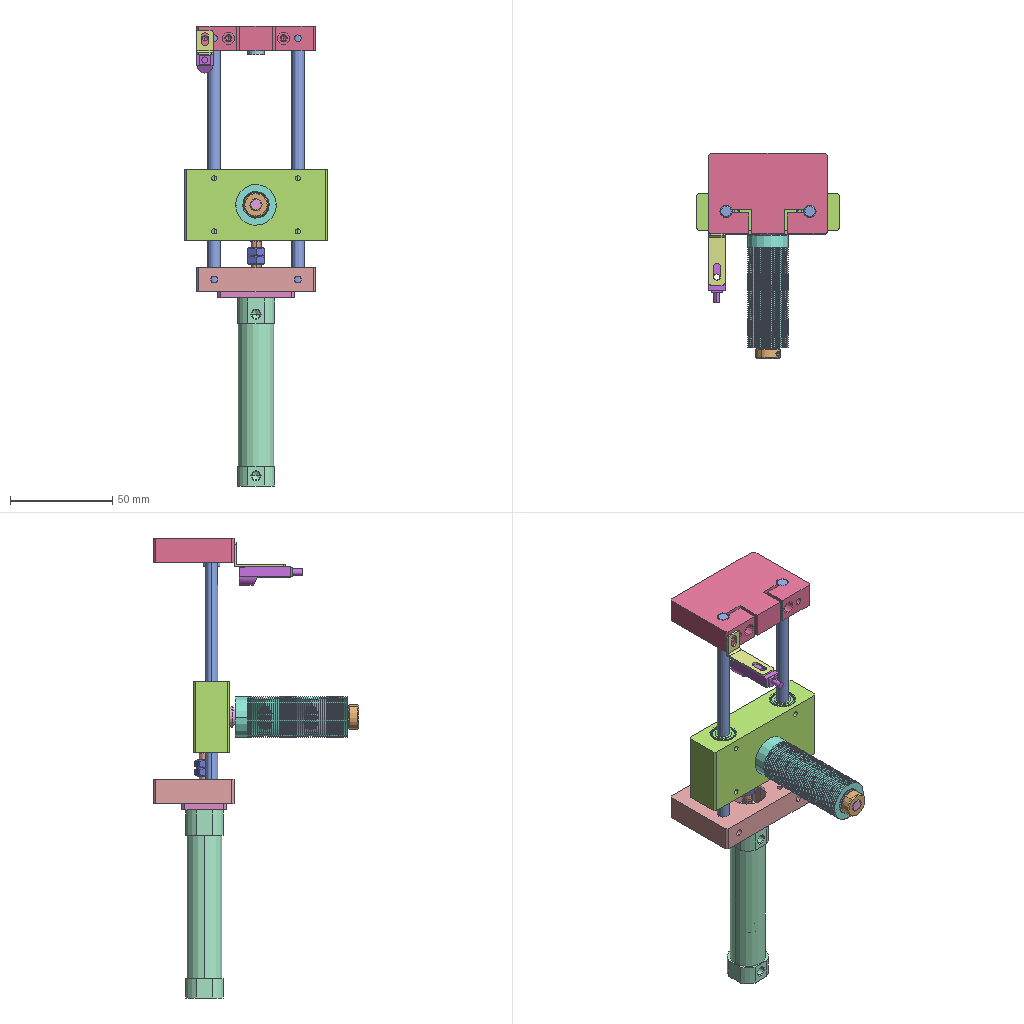Assembly | SolidWorks | 17 different items | 21 placed | box 70 x 100 x 225 mm
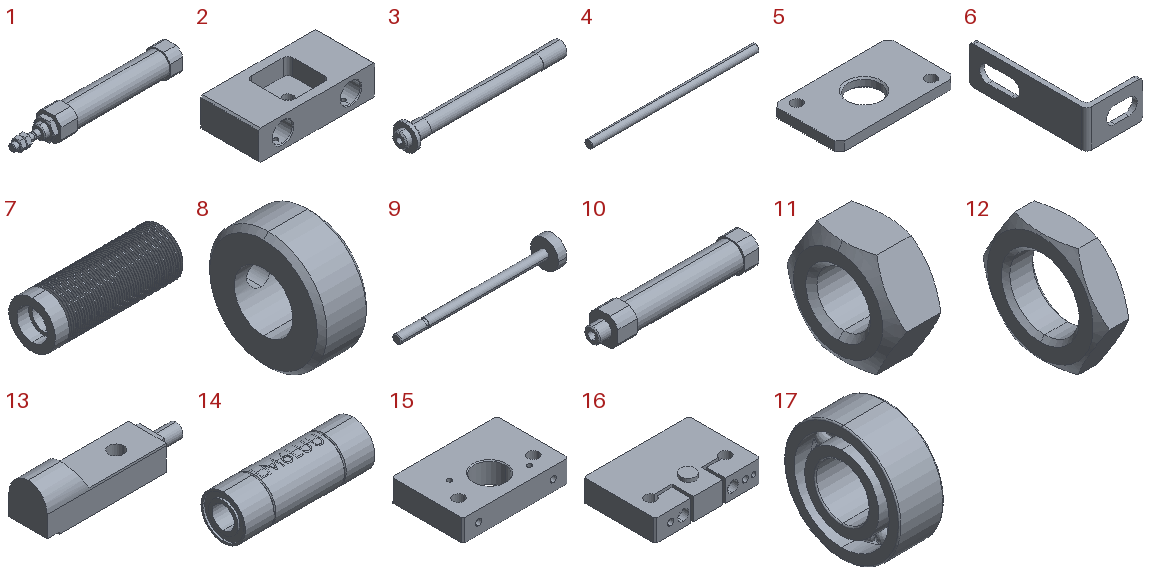Parts list (item | name | quantity | parent item | size | volume | features):
1 | (subassembly) | x1 | - | 120 x 18.3 x 18.3 mm | 16552 mm3 | -
2 | - | x1 | - | 70 x 35 x 18 mm | 29673 mm3 | features ICE 3, Chamfer 2, HoleWzd 2, Extrusion 1
3 | - | x1 | - | 65.5 x 10 x 10 mm | 1830 mm3 | features Chamfer 2, HoleWzd 1, Revolution 1
4 | - | x2 | - | 130 x 6 x 6 mm | 3671 mm3 | features Chamfer 1, Revolution 1
5 | - | x1 | - | 38 x 22 x 3 mm | 2168 mm3 | features Chamfer 2, Extrusion 1
6 | - | x1 | - | 12 x 25 x 8 mm | 239.899 mm3 | features ICE 2, ExtruThin 1, Fillet 1
7 | - | x1 | - | 55 x 20 x 20 mm | 10654 mm3 | features Revolution 1
8 | - | x1 | - | 5.5 x 12 x 12 mm | 411.056 mm3 | features Chamfer 1, HoleWzd 1, Revolution 1
9 | - | x1 | in 1 | 90.5 x 16 x 16 mm | 2673 mm3 | features RefAxis 12, 3DProfileFeature 4, Revolution 1
10 | - | x1 | in 1 | 100 x 18.3 x 18.3 mm | 13157 mm3 | features RefAxis 6, ICE 3, 3DProfileFeature 2, HoleWzd 2, RevCut 1, Revolution 1
11 | - | x2 | in 1 | 4 x 9.238 x 8 mm | 156.615 mm3 | features RefAxis 3, RevCut 2, 3DProfileFeature 1, Extrusion 1
12 | - | x1 | in 1 | 4 x 16.166 x 14 mm | 408.527 mm3 | features RefAxis 3, RevCut 2, 3DProfileFeature 1, Extrusion 1
13 | - | x1 | - | 31 x 8 x 9.093 mm | 1254 mm3 | features ICE 4, Extrusion 1, Fillet 1
14 | - | x2 | - | 35 x 12 x 12 mm | 2917 mm3 | features Emboss 1, Revolution 1
15 | - | x1 | - | 58 x 39.5 x 12 mm | 23617 mm3 | features Chamfer 2, HoleWzd 2, Extrusion 1, MirrorPattern 1
16 | - | x1 | - | 58 x 39.5 x 14 mm | 25416 mm3 | features HoleWzd 4, ICE 2, Chamfer 1, Extrusion 1, MirrorPattern 1
17 | - | x2 | - | 5 x 13 x 13 mm | 374.773 mm3 | features Stock 1
Mates (type | each side: item.copy, entity, surface, feature):
In the top assembly
Coincident | 15.1 face plane Boss-Extrude1 | 4.1 face plane Revolve1
Coincident | 15.1 face plane Boss-Extrude1 | 4.2 face plane Revolve1
Coincident | 2.1 face plane Boss-Extrude1 | 14.1 face plane Revolve1
Coincident | 2.1 face plane Boss-Extrude1 | 14.2 face plane Revolve1
Concentric | 4.1 face cylinder Revolve1 | 14.1 face cylinder Revolve1
Concentric | 4.2 face cylinder Revolve1 | 14.2 face cylinder Revolve1
Concentric | 7.1 face cylinder Revolve1 | 17.1 face cylinder 686ZZ Deep Groove Ball Bearing GB
Coincident | 7.1 face plane Revolve1 | 17.1 face plane 686ZZ Deep Groove Ball Bearing GB
Concentric | 7.1 face cylinder Revolve1 | 17.2 face cylinder 686ZZ Deep Groove Ball Bearing GB
Coincident | 7.1 face plane Revolve1 | 17.2 face plane 686ZZ Deep Groove Ball Bearing GB
Concentric | 3.1 face cylinder Revolve1 | 17.1 face cylinder 686ZZ Deep Groove Ball Bearing GB
Coincident | 3.1 face plane Revolve1 | 7.1 face plane Revolve1
Concentric | 3.1 face cylinder Revolve1 | 8.1 face cylinder Revolve1
Coincident | 8.1 face plane Revolve1 | 17.2 face plane 686ZZ Deep Groove Ball Bearing GB
Concentric | 4.1 face cylinder Revolve1 | 16.1 face cylinder Boss-Extrude1
Concentric | 4.2 face cylinder Revolve1 | 16.1 face cylinder Boss-Extrude1
Coincident | 4.2 face plane Revolve1 | 16.1 face plane Boss-Extrude1
Coincident | 16.1 face plane Boss-Extrude1 | 6.1 face plane Extrude-Thin1 | 2 times
DistanceDim | 16.1 face plane Boss-Extrude1 | 6.1 face plane Extrude-Thin1
Coincident | 6.1 face plane Extrude-Thin1 | 13.1 face plane Boss-Extrude1 | 2 times
Concentric | 15.1 face cylinder Boss-Extrude1 | 4.2 face cylinder Revolve1
Concentric | 15.1 face cylinder Boss-Extrude1 | 4.1 face cylinder Revolve1
Concentric | 2.1 face cylinder Cut-Extrude2 | 14.2 face cylinder Revolve1
Concentric | 2.1 face cylinder Cut-Extrude2 | 14.1 face cylinder Revolve1
Coincident | 2.1 face plane Boss-Extrude1 | 3.1 face plane Revolve1
Concentric | 10.1 face cylinder Revolve1 | 5.1 face cylinder Boss-Extrude1
Coincident | 10.1 face plane Boss-Extrude1 | 5.1 face plane Boss-Extrude1
Coincident | 15.1 face plane Boss-Extrude1 | 5.1 face plane Boss-Extrude1
Concentric | 15.1 face cylinder M3 Tapped Hole1 | 5.1 face cylinder Boss-Extrude1 | 2 times
LimitDistanceDim | 2.1 face plane Boss-Extrude1 | 9.1 face plane Revolve1
Concentric | 2.1 face cylinder Cut-Extrude3 | 3.1 face cylinder Revolve1
Parallel | 15.1 face plane Boss-Extrude1 | 10.1 face plane Boss-Extrude1
In subassembly 1
Coincident | 10.2 axis | 9.2 axis
PlanarAngleDim | 9.2 plane | 10.2 plane
Coincident | 9.2 axis | 11.1 axis
DistanceDim | 11.2 plane | 9.2 plane
Coincident | 9.2 axis | 11.2 axis
PlanarAngleDim | 11.2 plane | 9.2 plane